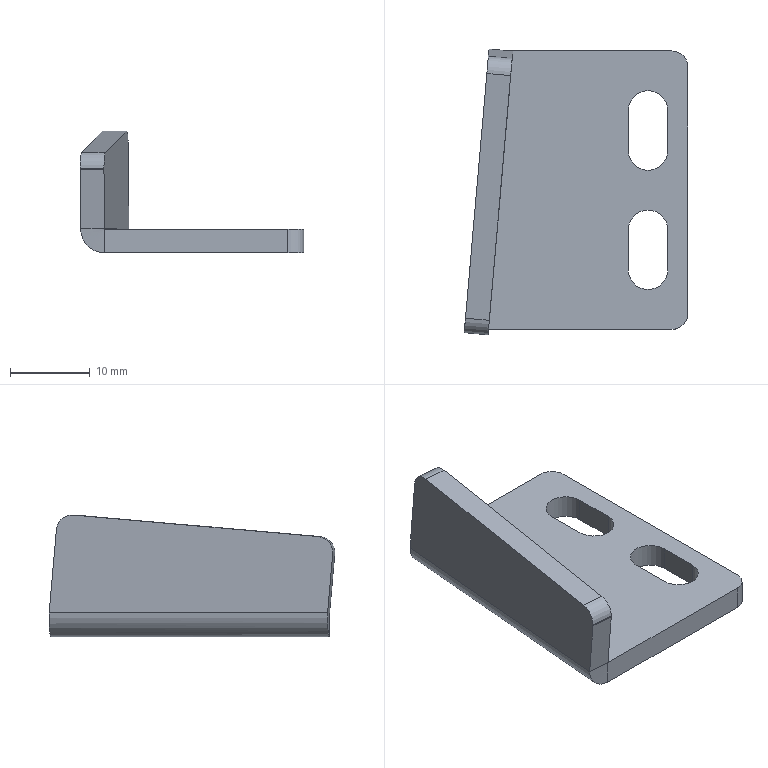Part | NX | features BREP 1 | 1 solid | 27 faces | box 28.112 x 35.918 x 15.317 mm | volume 3596 mm3 | plane 14 | cylinder 11 | spline 2 | commonest cylinder face diameters 4 x5 5 x4 0.02 x1 6.02 x1
STEP:
#1=CARTESIAN_POINT('',(-7.623,-18.197,10.615));
#2=VERTEX_POINT('',#1);
#3=CARTESIAN_POINT('',(-7.622,-18.189,10.441));
#4=VERTEX_POINT('',#3);
#5=CARTESIAN_POINT('',(-7.449,-16.204,10.615));
#6=DIRECTION('',(0.9962,-0.08716,0.));
#7=DIRECTION('',(0.08716,0.9962,0.));
#8=AXIS2_PLACEMENT_3D('',#5,#6,#7);
#9=CIRCLE('',#8,2.);
#10=EDGE_CURVE('',#2,#4,#9,.T.);
#11=ORIENTED_EDGE('',*,*,#10,.F.);
#12=CARTESIAN_POINT('',(-10.612,-17.935,10.615));
#13=VERTEX_POINT('',#12);
#14=CARTESIAN_POINT('',(-7.623,-18.197,10.615));
#15=DIRECTION('',(-0.9962,0.08716,0.));
#16=VECTOR('',#15,1000.);
#17=LINE('',#14,#16);
#18=EDGE_CURVE('',#2,#13,#17,.T.);
#19=ORIENTED_EDGE('',*,*,#18,.T.);
#20=CARTESIAN_POINT('',(-10.611,-17.928,10.441));
#21=VERTEX_POINT('',#20);
#22=CARTESIAN_POINT('',(-10.437,-15.943,10.615));
#23=DIRECTION('',(-0.9962,0.08716,0.));
#24=DIRECTION('',(0.08716,0.9962,0.));
#25=AXIS2_PLACEMENT_3D('',#22,#23,#24);
#26=CIRCLE('',#25,2.);
#27=EDGE_CURVE('',#21,#13,#26,.T.);
#28=ORIENTED_EDGE('',*,*,#27,.F.);
#29=CARTESIAN_POINT('',(-7.622,-18.189,10.441));
#30=DIRECTION('',(-0.9962,0.08716,0.));
#31=VECTOR('',#30,1000.);
#32=LINE('',#29,#31);
#33=EDGE_CURVE('',#4,#21,#32,.T.);
#34=ORIENTED_EDGE('',*,*,#33,.F.);
#35=EDGE_LOOP('',(#11,#19,#28,#34));
#36=FACE_BOUND('',#35,.T.);
#37=CARTESIAN_POINT('',(-7.449,-16.204,10.615));
#38=DIRECTION('',(-0.9962,0.08716,0.));
#39=DIRECTION('',(-0.08716,-0.9962,0.));
#40=AXIS2_PLACEMENT_3D('',#37,#38,#39);
#41=CYLINDRICAL_SURFACE('',#40,2.);
#42=ADVANCED_FACE('',(#36),#41,.T.);
#43=CARTESIAN_POINT('',(-4.504,17.458,3.01));
#44=VERTEX_POINT('',#43);
#45=CARTESIAN_POINT('',(-4.584,16.545,13.491));
#46=VERTEX_POINT('',#45);
#47=CARTESIAN_POINT('',(-4.599,16.371,15.484));
#48=DIRECTION('',(-0.007596,-0.08682,0.9962));
#49=VECTOR('',#48,1000.);
#50=LINE('',#47,#49);
#51=EDGE_CURVE('',#44,#46,#50,.T.);
#52=ORIENTED_EDGE('',*,*,#51,.T.);
#53=CARTESIAN_POINT('',(-4.772,14.386,15.309));
#54=VERTEX_POINT('',#53);
#55=CARTESIAN_POINT('',(-4.757,14.56,13.317));
#56=DIRECTION('',(0.9962,-0.08716,0.));
#57=DIRECTION('',(0.08716,0.9962,0.));
#58=AXIS2_PLACEMENT_3D('',#55,#56,#57);
#59=CIRCLE('',#58,2.);
#60=EDGE_CURVE('',#46,#54,#59,.T.);
#61=ORIENTED_EDGE('',*,*,#60,.T.);
#62=CARTESIAN_POINT('',(-7.464,-16.378,12.607));
#63=VERTEX_POINT('',#62);
#64=CARTESIAN_POINT('',(-4.599,16.371,15.484));
#65=DIRECTION('',(-0.08682,-0.9924,-0.08716));
#66=VECTOR('',#65,1000.);
#67=LINE('',#64,#66);
#68=EDGE_CURVE('',#54,#63,#67,.T.);
#69=ORIENTED_EDGE('',*,*,#68,.T.);
#70=CARTESIAN_POINT('',(-7.449,-16.204,10.615));
#71=DIRECTION('',(0.9962,-0.08716,0.));
#72=DIRECTION('',(0.08716,0.9962,0.));
#73=AXIS2_PLACEMENT_3D('',#70,#71,#72);
#74=CIRCLE('',#73,2.);
#75=EDGE_CURVE('',#63,#2,#74,.T.);
#76=ORIENTED_EDGE('',*,*,#75,.T.);
#77=ORIENTED_EDGE('',*,*,#10,.T.);
#78=CARTESIAN_POINT('',(-7.566,-17.542,3.01));
#79=VERTEX_POINT('',#78);
#80=CARTESIAN_POINT('',(-7.638,-18.363,12.433));
#81=DIRECTION('',(0.007596,0.08682,-0.9962));
#82=VECTOR('',#81,1000.);
#83=LINE('',#80,#82);
#84=EDGE_CURVE('',#4,#79,#83,.T.);
#85=ORIENTED_EDGE('',*,*,#84,.T.);
#86=CARTESIAN_POINT('',(-7.638,-18.363,3.01));
#87=DIRECTION('',(0.08716,0.9962,0.));
#88=VECTOR('',#87,1000.);
#89=LINE('',#86,#88);
#90=EDGE_CURVE('',#79,#44,#89,.T.);
#91=ORIENTED_EDGE('',*,*,#90,.T.);
#92=EDGE_LOOP('',(#52,#61,#69,#76,#77,#85,#91));
#93=FACE_BOUND('',#92,.T.);
#94=CARTESIAN_POINT('',(-7.638,-18.363,12.433));
#95=DIRECTION('',(0.9962,-0.08716,0.));
#96=DIRECTION('',(0.,0.,-1.));
#97=AXIS2_PLACEMENT_3D('',#94,#95,#96);
#98=PLANE('',#97);
#99=ADVANCED_FACE('',(#93),#98,.T.);
#100=ORIENTED_EDGE('',*,*,#68,.F.);
#101=CARTESIAN_POINT('',(-7.761,14.648,15.309));
#102=VERTEX_POINT('',#101);
#103=CARTESIAN_POINT('',(-4.772,14.386,15.309));
#104=DIRECTION('',(-0.9962,0.08716,0.));
#105=VECTOR('',#104,1000.);
#106=LINE('',#103,#105);
#107=EDGE_CURVE('',#54,#102,#106,.T.);
#108=ORIENTED_EDGE('',*,*,#107,.T.);
#109=CARTESIAN_POINT('',(-10.453,-16.117,12.607));
#110=VERTEX_POINT('',#109);
#111=CARTESIAN_POINT('',(-7.587,16.633,15.484));
#112=DIRECTION('',(-0.08682,-0.9924,-0.08716));
#113=VECTOR('',#112,1000.);
#114=LINE('',#111,#113);
#115=EDGE_CURVE('',#102,#110,#114,.T.);
#116=ORIENTED_EDGE('',*,*,#115,.T.);
#117=CARTESIAN_POINT('',(-7.464,-16.378,12.607));
#118=DIRECTION('',(0.9962,-0.08716,0.));
#119=VECTOR('',#118,1000.);
#120=LINE('',#117,#119);
#121=EDGE_CURVE('',#110,#63,#120,.T.);
#122=ORIENTED_EDGE('',*,*,#121,.T.);
#123=EDGE_LOOP('',(#100,#108,#116,#122));
#124=FACE_BOUND('',#123,.T.);
#125=CARTESIAN_POINT('',(-4.599,16.371,15.484));
#126=DIRECTION('',(0.007596,0.08682,-0.9962));
#127=DIRECTION('',(-1.,0.,-0.007625));
#128=AXIS2_PLACEMENT_3D('',#125,#126,#127);
#129=PLANE('',#128);
#130=ADVANCED_FACE('',(#124),#129,.F.);
#131=ORIENTED_EDGE('',*,*,#84,.F.);
#132=ORIENTED_EDGE('',*,*,#33,.T.);
#133=CARTESIAN_POINT('',(-10.554,-17.28,3.01));
#134=VERTEX_POINT('',#133);
#135=CARTESIAN_POINT('',(-10.626,-18.101,12.433));
#136=DIRECTION('',(0.007596,0.08682,-0.9962));
#137=VECTOR('',#136,1000.);
#138=LINE('',#135,#137);
#139=EDGE_CURVE('',#21,#134,#138,.T.);
#140=ORIENTED_EDGE('',*,*,#139,.T.);
#141=CARTESIAN_POINT('',(-7.566,-17.542,3.01));
#142=CARTESIAN_POINT('',(-10.554,-17.28,3.01));
#143=B_SPLINE_CURVE_WITH_KNOTS('',1,(#141,#142),.UNSPECIFIED.,.F.,.F.,(2,2),(0.,1.),.UNSPECIFIED.);
#144=EDGE_CURVE('',#79,#134,#143,.T.);
#145=ORIENTED_EDGE('',*,*,#144,.F.);
#146=EDGE_LOOP('',(#131,#132,#140,#145));
#147=FACE_BOUND('',#146,.T.);
#148=CARTESIAN_POINT('',(-7.638,-18.363,12.433));
#149=DIRECTION('',(0.08682,0.9924,0.08716));
#150=DIRECTION('',(0.7085,0.,-0.7058));
#151=AXIS2_PLACEMENT_3D('',#148,#149,#150);
#152=PLANE('',#151);
#153=ADVANCED_FACE('',(#147),#152,.F.);
#154=CARTESIAN_POINT('',(-7.492,17.72,3.01));
#155=VERTEX_POINT('',#154);
#156=CARTESIAN_POINT('',(-7.572,16.806,13.491));
#157=VERTEX_POINT('',#156);
#158=CARTESIAN_POINT('',(-7.587,16.633,15.484));
#159=DIRECTION('',(-0.007596,-0.08682,0.9962));
#160=VECTOR('',#159,1000.);
#161=LINE('',#158,#160);
#162=EDGE_CURVE('',#155,#157,#161,.T.);
#163=ORIENTED_EDGE('',*,*,#162,.T.);
#164=CARTESIAN_POINT('',(-4.584,16.545,13.491));
#165=DIRECTION('',(0.9962,-0.08716,0.));
#166=VECTOR('',#165,1000.);
#167=LINE('',#164,#166);
#168=EDGE_CURVE('',#157,#46,#167,.T.);
#169=ORIENTED_EDGE('',*,*,#168,.T.);
#170=ORIENTED_EDGE('',*,*,#51,.F.);
#171=CARTESIAN_POINT('',(-7.492,17.72,3.01));
#172=CARTESIAN_POINT('',(-4.504,17.458,3.01));
#173=B_SPLINE_CURVE_WITH_KNOTS('',1,(#171,#172),.UNSPECIFIED.,.F.,.F.,(2,2),(0.,1.),.UNSPECIFIED.);
#174=EDGE_CURVE('',#155,#44,#173,.T.);
#175=ORIENTED_EDGE('',*,*,#174,.F.);
#176=EDGE_LOOP('',(#163,#169,#170,#175));
#177=FACE_BOUND('',#176,.T.);
#178=CARTESIAN_POINT('',(-4.599,16.371,15.484));
#179=DIRECTION('',(-0.08682,-0.9924,-0.08716));
#180=DIRECTION('',(0.,0.08749,-0.9962));
#181=AXIS2_PLACEMENT_3D('',#178,#179,#180);
#182=PLANE('',#181);
#183=ADVANCED_FACE('',(#177),#182,.F.);
#184=ORIENTED_EDGE('',*,*,#115,.F.);
#185=CARTESIAN_POINT('',(-7.746,14.822,13.317));
#186=DIRECTION('',(-0.9962,0.08716,0.));
#187=DIRECTION('',(0.08716,0.9962,0.));
#188=AXIS2_PLACEMENT_3D('',#185,#186,#187);
#189=CIRCLE('',#188,2.);
#190=EDGE_CURVE('',#102,#157,#189,.T.);
#191=ORIENTED_EDGE('',*,*,#190,.T.);
#192=ORIENTED_EDGE('',*,*,#162,.F.);
#193=CARTESIAN_POINT('',(-10.626,-18.101,3.01));
#194=DIRECTION('',(0.08716,0.9962,0.));
#195=VECTOR('',#194,1000.);
#196=LINE('',#193,#195);
#197=EDGE_CURVE('',#134,#155,#196,.T.);
#198=ORIENTED_EDGE('',*,*,#197,.F.);
#199=ORIENTED_EDGE('',*,*,#139,.F.);
#200=ORIENTED_EDGE('',*,*,#27,.T.);
#201=CARTESIAN_POINT('',(-10.437,-15.943,10.615));
#202=DIRECTION('',(-0.9962,0.08716,0.));
#203=DIRECTION('',(0.08716,0.9962,0.));
#204=AXIS2_PLACEMENT_3D('',#201,#202,#203);
#205=CIRCLE('',#204,2.);
#206=EDGE_CURVE('',#13,#110,#205,.T.);
#207=ORIENTED_EDGE('',*,*,#206,.T.);
#208=EDGE_LOOP('',(#184,#191,#192,#198,#199,#200,#207));
#209=FACE_BOUND('',#208,.T.);
#210=CARTESIAN_POINT('',(-10.626,-18.101,12.433));
#211=DIRECTION('',(0.9962,-0.08716,0.));
#212=DIRECTION('',(0.,0.,-1.));
#213=AXIS2_PLACEMENT_3D('',#210,#211,#212);
#214=PLANE('',#213);
#215=ADVANCED_FACE('',(#209),#214,.F.);
#216=CARTESIAN_POINT('',(17.5,-15.5,3.));
#217=VERTEX_POINT('',#216);
#218=CARTESIAN_POINT('',(17.5,15.5,3.));
#219=VERTEX_POINT('',#218);
#220=CARTESIAN_POINT('',(17.5,17.5,3.));
#221=DIRECTION('',(0.,1.,0.));
#222=VECTOR('',#221,1000.);
#223=LINE('',#220,#222);
#224=EDGE_CURVE('',#217,#219,#223,.T.);
#225=ORIENTED_EDGE('',*,*,#224,.F.);
#226=CARTESIAN_POINT('',(17.5,-15.5,0.));
#227=VERTEX_POINT('',#226);
#228=CARTESIAN_POINT('',(17.5,-15.5,3.));
#229=DIRECTION('',(0.,0.,-1.));
#230=VECTOR('',#229,1000.);
#231=LINE('',#228,#230);
#232=EDGE_CURVE('',#217,#227,#231,.T.);
#233=ORIENTED_EDGE('',*,*,#232,.T.);
#234=CARTESIAN_POINT('',(17.5,15.5,0.));
#235=VERTEX_POINT('',#234);
#236=CARTESIAN_POINT('',(17.5,17.5,0.));
#237=DIRECTION('',(0.,1.,0.));
#238=VECTOR('',#237,1000.);
#239=LINE('',#236,#238);
#240=EDGE_CURVE('',#227,#235,#239,.T.);
#241=ORIENTED_EDGE('',*,*,#240,.T.);
#242=CARTESIAN_POINT('',(17.5,15.5,3.));
#243=DIRECTION('',(0.,0.,1.));
#244=VECTOR('',#243,1000.);
#245=LINE('',#242,#244);
#246=EDGE_CURVE('',#235,#219,#245,.T.);
#247=ORIENTED_EDGE('',*,*,#246,.T.);
#248=EDGE_LOOP('',(#225,#233,#241,#247));
#249=FACE_BOUND('',#248,.T.);
#250=CARTESIAN_POINT('',(17.5,17.5,3.));
#251=DIRECTION('',(-1.,0.,0.));
#252=DIRECTION('',(0.,1.,0.));
#253=AXIS2_PLACEMENT_3D('',#250,#251,#252);
#254=PLANE('',#253);
#255=ADVANCED_FACE('',(#249),#254,.F.);
#256=CARTESIAN_POINT('',(-7.552,-17.5,3.));
#257=VERTEX_POINT('',#256);
#258=CARTESIAN_POINT('',(15.5,-17.5,3.));
#259=VERTEX_POINT('',#258);
#260=CARTESIAN_POINT('',(-17.5,-17.5,3.));
#261=DIRECTION('',(1.,0.,0.));
#262=VECTOR('',#261,1000.);
#263=LINE('',#260,#262);
#264=EDGE_CURVE('',#257,#259,#263,.T.);
#265=ORIENTED_EDGE('',*,*,#264,.T.);
#266=CARTESIAN_POINT('',(15.5,-15.5,3.));
#267=DIRECTION('',(0.,0.,1.));
#268=DIRECTION('',(1.,0.,0.));
#269=AXIS2_PLACEMENT_3D('',#266,#267,#268);
#270=CIRCLE('',#269,2.);
#271=EDGE_CURVE('',#259,#217,#270,.T.);
#272=ORIENTED_EDGE('',*,*,#271,.T.);
#273=ORIENTED_EDGE('',*,*,#224,.T.);
#274=CARTESIAN_POINT('',(15.5,17.5,3.));
#275=VERTEX_POINT('',#274);
#276=CARTESIAN_POINT('',(15.5,15.5,3.));
#277=DIRECTION('',(0.,0.,1.));
#278=DIRECTION('',(1.,0.,0.));
#279=AXIS2_PLACEMENT_3D('',#276,#277,#278);
#280=CIRCLE('',#279,2.);
#281=EDGE_CURVE('',#219,#275,#280,.T.);
#282=ORIENTED_EDGE('',*,*,#281,.T.);
#283=CARTESIAN_POINT('',(-4.49,17.5,3.));
#284=VERTEX_POINT('',#283);
#285=CARTESIAN_POINT('',(-17.5,17.5,3.));
#286=DIRECTION('',(-1.,0.,0.));
#287=VECTOR('',#286,1000.);
#288=LINE('',#285,#287);
#289=EDGE_CURVE('',#275,#284,#288,.T.);
#290=ORIENTED_EDGE('',*,*,#289,.T.);
#291=CARTESIAN_POINT('',(-7.628,-18.364,3.));
#292=DIRECTION('',(0.08716,0.9962,0.));
#293=VECTOR('',#292,1000.);
#294=LINE('',#291,#293);
#295=EDGE_CURVE('',#257,#284,#294,.T.);
#296=ORIENTED_EDGE('',*,*,#295,.F.);
#297=EDGE_LOOP('',(#265,#272,#273,#282,#290,#296));
#298=FACE_BOUND('',#297,.T.);
#299=CARTESIAN_POINT('',(15.,-5.,3.));
#300=VERTEX_POINT('',#299);
#301=CARTESIAN_POINT('',(10.,-5.,3.));
#302=VERTEX_POINT('',#301);
#303=CARTESIAN_POINT('',(12.5,-5.,3.));
#304=DIRECTION('',(0.,0.,1.));
#305=DIRECTION('',(-1.,0.,0.));
#306=AXIS2_PLACEMENT_3D('',#303,#304,#305);
#307=CIRCLE('',#306,2.5);
#308=EDGE_CURVE('',#300,#302,#307,.T.);
#309=ORIENTED_EDGE('',*,*,#308,.F.);
#310=CARTESIAN_POINT('',(15.,-10.,3.));
#311=VERTEX_POINT('',#310);
#312=CARTESIAN_POINT('',(15.,-5.,3.));
#313=DIRECTION('',(0.,1.,0.));
#314=VECTOR('',#313,1000.);
#315=LINE('',#312,#314);
#316=EDGE_CURVE('',#311,#300,#315,.T.);
#317=ORIENTED_EDGE('',*,*,#316,.F.);
#318=CARTESIAN_POINT('',(10.,-10.,3.));
#319=VERTEX_POINT('',#318);
#320=CARTESIAN_POINT('',(12.5,-10.,3.));
#321=DIRECTION('',(0.,0.,1.));
#322=DIRECTION('',(-1.,0.,0.));
#323=AXIS2_PLACEMENT_3D('',#320,#321,#322);
#324=CIRCLE('',#323,2.5);
#325=EDGE_CURVE('',#319,#311,#324,.T.);
#326=ORIENTED_EDGE('',*,*,#325,.F.);
#327=CARTESIAN_POINT('',(10.,-10.,3.));
#328=DIRECTION('',(0.,-1.,0.));
#329=VECTOR('',#328,1000.);
#330=LINE('',#327,#329);
#331=EDGE_CURVE('',#302,#319,#330,.T.);
#332=ORIENTED_EDGE('',*,*,#331,.F.);
#333=EDGE_LOOP('',(#309,#317,#326,#332));
#334=FACE_BOUND('',#333,.T.);
#335=CARTESIAN_POINT('',(15.,10.,3.));
#336=VERTEX_POINT('',#335);
#337=CARTESIAN_POINT('',(10.,10.,3.));
#338=VERTEX_POINT('',#337);
#339=CARTESIAN_POINT('',(12.5,10.,3.));
#340=DIRECTION('',(0.,0.,1.));
#341=DIRECTION('',(-1.,0.,0.));
#342=AXIS2_PLACEMENT_3D('',#339,#340,#341);
#343=CIRCLE('',#342,2.5);
#344=EDGE_CURVE('',#336,#338,#343,.T.);
#345=ORIENTED_EDGE('',*,*,#344,.F.);
#346=CARTESIAN_POINT('',(15.,5.,3.));
#347=VERTEX_POINT('',#346);
#348=CARTESIAN_POINT('',(15.,10.,3.));
#349=DIRECTION('',(0.,1.,0.));
#350=VECTOR('',#349,1000.);
#351=LINE('',#348,#350);
#352=EDGE_CURVE('',#347,#336,#351,.T.);
#353=ORIENTED_EDGE('',*,*,#352,.F.);
#354=CARTESIAN_POINT('',(10.,5.,3.));
#355=VERTEX_POINT('',#354);
#356=CARTESIAN_POINT('',(12.5,5.,3.));
#357=DIRECTION('',(0.,0.,1.));
#358=DIRECTION('',(-1.,0.,0.));
#359=AXIS2_PLACEMENT_3D('',#356,#357,#358);
#360=CIRCLE('',#359,2.5);
#361=EDGE_CURVE('',#355,#347,#360,.T.);
#362=ORIENTED_EDGE('',*,*,#361,.F.);
#363=CARTESIAN_POINT('',(10.,5.,3.));
#364=DIRECTION('',(0.,-1.,0.));
#365=VECTOR('',#364,1000.);
#366=LINE('',#363,#365);
#367=EDGE_CURVE('',#338,#355,#366,.T.);
#368=ORIENTED_EDGE('',*,*,#367,.F.);
#369=EDGE_LOOP('',(#345,#353,#362,#368));
#370=FACE_BOUND('',#369,.T.);
#371=CARTESIAN_POINT('',(-17.5,-17.5,3.));
#372=DIRECTION('',(0.,0.,1.));
#373=DIRECTION('',(1.,0.,0.));
#374=AXIS2_PLACEMENT_3D('',#371,#372,#373);
#375=PLANE('',#374);
#376=ADVANCED_FACE('',(#298,#334,#370),#375,.T.);
#377=CARTESIAN_POINT('',(-7.552,-17.5,0.));
#378=VERTEX_POINT('',#377);
#379=CARTESIAN_POINT('',(15.5,-17.5,0.));
#380=VERTEX_POINT('',#379);
#381=CARTESIAN_POINT('',(-17.5,-17.5,0.));
#382=DIRECTION('',(1.,0.,0.));
#383=VECTOR('',#382,1000.);
#384=LINE('',#381,#383);
#385=EDGE_CURVE('',#378,#380,#384,.T.);
#386=ORIENTED_EDGE('',*,*,#385,.T.);
#387=CARTESIAN_POINT('',(15.5,-17.5,3.));
#388=DIRECTION('',(0.,0.,1.));
#389=VECTOR('',#388,1000.);
#390=LINE('',#387,#389);
#391=EDGE_CURVE('',#380,#259,#390,.T.);
#392=ORIENTED_EDGE('',*,*,#391,.T.);
#393=ORIENTED_EDGE('',*,*,#264,.F.);
#394=CARTESIAN_POINT('',(-7.552,-17.5,3.));
#395=CARTESIAN_POINT('',(-7.552,-17.5,2.));
#396=CARTESIAN_POINT('',(-7.552,-17.5,1.));
#397=CARTESIAN_POINT('',(-7.552,-17.5,0.));
#398=B_SPLINE_CURVE_WITH_KNOTS('',3,(#394,#395,#396,#397),.UNSPECIFIED.,.F.,.F.,(4,4),(0.,1.),.UNSPECIFIED.);
#399=EDGE_CURVE('',#257,#378,#398,.T.);
#400=ORIENTED_EDGE('',*,*,#399,.T.);
#401=EDGE_LOOP('',(#386,#392,#393,#400));
#402=FACE_BOUND('',#401,.T.);
#403=CARTESIAN_POINT('',(-17.5,-17.5,3.));
#404=DIRECTION('',(0.,1.,0.));
#405=DIRECTION('',(1.,0.,0.));
#406=AXIS2_PLACEMENT_3D('',#403,#404,#405);
#407=PLANE('',#406);
#408=ADVANCED_FACE('',(#402),#407,.F.);
#409=ORIENTED_EDGE('',*,*,#240,.F.);
#410=CARTESIAN_POINT('',(15.5,-15.5,0.));
#411=DIRECTION('',(0.,0.,-1.));
#412=DIRECTION('',(1.,0.,0.));
#413=AXIS2_PLACEMENT_3D('',#410,#411,#412);
#414=CIRCLE('',#413,2.);
#415=EDGE_CURVE('',#227,#380,#414,.T.);
#416=ORIENTED_EDGE('',*,*,#415,.T.);
#417=ORIENTED_EDGE('',*,*,#385,.F.);
#418=CARTESIAN_POINT('',(-4.49,17.5,-0.000000004));
#419=VERTEX_POINT('',#418);
#420=CARTESIAN_POINT('',(-7.628,-18.364,0.));
#421=DIRECTION('',(0.08716,0.9962,0.));
#422=VECTOR('',#421,1000.);
#423=LINE('',#420,#422);
#424=EDGE_CURVE('',#378,#419,#423,.T.);
#425=ORIENTED_EDGE('',*,*,#424,.T.);
#426=CARTESIAN_POINT('',(15.5,17.5,0.));
#427=VERTEX_POINT('',#426);
#428=CARTESIAN_POINT('',(-17.5,17.5,0.));
#429=DIRECTION('',(-1.,0.,0.));
#430=VECTOR('',#429,1000.);
#431=LINE('',#428,#430);
#432=EDGE_CURVE('',#427,#419,#431,.T.);
#433=ORIENTED_EDGE('',*,*,#432,.F.);
#434=CARTESIAN_POINT('',(15.5,15.5,0.));
#435=DIRECTION('',(0.,0.,-1.));
#436=DIRECTION('',(1.,0.,0.));
#437=AXIS2_PLACEMENT_3D('',#434,#435,#436);
#438=CIRCLE('',#437,2.);
#439=EDGE_CURVE('',#427,#235,#438,.T.);
#440=ORIENTED_EDGE('',*,*,#439,.T.);
#441=EDGE_LOOP('',(#409,#416,#417,#425,#433,#440));
#442=FACE_BOUND('',#441,.T.);
#443=CARTESIAN_POINT('',(15.,-10.,0.));
#444=VERTEX_POINT('',#443);
#445=CARTESIAN_POINT('',(15.,-5.,0.));
#446=VERTEX_POINT('',#445);
#447=CARTESIAN_POINT('',(15.,-17.5,0.));
#448=DIRECTION('',(0.,1.,0.));
#449=VECTOR('',#448,1000.);
#450=LINE('',#447,#449);
#451=EDGE_CURVE('',#444,#446,#450,.T.);
#452=ORIENTED_EDGE('',*,*,#451,.T.);
#453=CARTESIAN_POINT('',(10.,-5.,0.));
#454=VERTEX_POINT('',#453);
#455=CARTESIAN_POINT('',(12.5,-5.,0.));
#456=DIRECTION('',(0.,0.,1.));
#457=DIRECTION('',(1.,0.,0.));
#458=AXIS2_PLACEMENT_3D('',#455,#456,#457);
#459=CIRCLE('',#458,2.5);
#460=EDGE_CURVE('',#446,#454,#459,.T.);
#461=ORIENTED_EDGE('',*,*,#460,.T.);
#462=CARTESIAN_POINT('',(10.,-10.,0.));
#463=VERTEX_POINT('',#462);
#464=CARTESIAN_POINT('',(10.,-17.5,0.));
#465=DIRECTION('',(0.,-1.,0.));
#466=VECTOR('',#465,1000.);
#467=LINE('',#464,#466);
#468=EDGE_CURVE('',#454,#463,#467,.T.);
#469=ORIENTED_EDGE('',*,*,#468,.T.);
#470=CARTESIAN_POINT('',(12.5,-10.,0.));
#471=DIRECTION('',(0.,0.,1.));
#472=DIRECTION('',(1.,0.,0.));
#473=AXIS2_PLACEMENT_3D('',#470,#471,#472);
#474=CIRCLE('',#473,2.5);
#475=EDGE_CURVE('',#463,#444,#474,.T.);
#476=ORIENTED_EDGE('',*,*,#475,.T.);
#477=EDGE_LOOP('',(#452,#461,#469,#476));
#478=FACE_BOUND('',#477,.T.);
#479=CARTESIAN_POINT('',(15.,5.,0.));
#480=VERTEX_POINT('',#479);
#481=CARTESIAN_POINT('',(15.,10.,0.));
#482=VERTEX_POINT('',#481);
#483=CARTESIAN_POINT('',(15.,-17.5,0.));
#484=DIRECTION('',(0.,1.,0.));
#485=VECTOR('',#484,1000.);
#486=LINE('',#483,#485);
#487=EDGE_CURVE('',#480,#482,#486,.T.);
#488=ORIENTED_EDGE('',*,*,#487,.T.);
#489=CARTESIAN_POINT('',(10.,10.,0.));
#490=VERTEX_POINT('',#489);
#491=CARTESIAN_POINT('',(12.5,10.,0.));
#492=DIRECTION('',(0.,0.,1.));
#493=DIRECTION('',(1.,0.,0.));
#494=AXIS2_PLACEMENT_3D('',#491,#492,#493);
#495=CIRCLE('',#494,2.5);
#496=EDGE_CURVE('',#482,#490,#495,.T.);
#497=ORIENTED_EDGE('',*,*,#496,.T.);
#498=CARTESIAN_POINT('',(10.,5.,0.));
#499=VERTEX_POINT('',#498);
#500=CARTESIAN_POINT('',(10.,-17.5,0.));
#501=DIRECTION('',(0.,-1.,0.));
#502=VECTOR('',#501,1000.);
#503=LINE('',#500,#502);
#504=EDGE_CURVE('',#490,#499,#503,.T.);
#505=ORIENTED_EDGE('',*,*,#504,.T.);
#506=CARTESIAN_POINT('',(12.5,5.,0.));
#507=DIRECTION('',(0.,0.,1.));
#508=DIRECTION('',(1.,0.,0.));
#509=AXIS2_PLACEMENT_3D('',#506,#507,#508);
#510=CIRCLE('',#509,2.5);
#511=EDGE_CURVE('',#499,#480,#510,.T.);
#512=ORIENTED_EDGE('',*,*,#511,.T.);
#513=EDGE_LOOP('',(#488,#497,#505,#512));
#514=FACE_BOUND('',#513,.T.);
#515=CARTESIAN_POINT('',(-17.5,-17.5,0.));
#516=DIRECTION('',(0.,0.,1.));
#517=DIRECTION('',(1.,0.,0.));
#518=AXIS2_PLACEMENT_3D('',#515,#516,#517);
#519=PLANE('',#518);
#520=ADVANCED_FACE('',(#442,#478,#514),#519,.F.);
#521=ORIENTED_EDGE('',*,*,#289,.F.);
#522=CARTESIAN_POINT('',(15.5,17.5,3.));
#523=DIRECTION('',(0.,0.,-1.));
#524=VECTOR('',#523,1000.);
#525=LINE('',#522,#524);
#526=EDGE_CURVE('',#275,#427,#525,.T.);
#527=ORIENTED_EDGE('',*,*,#526,.T.);
#528=ORIENTED_EDGE('',*,*,#432,.T.);
#529=CARTESIAN_POINT('',(-4.49,17.5,-0.000000004));
#530=CARTESIAN_POINT('',(-4.49,17.5,1.));
#531=CARTESIAN_POINT('',(-4.49,17.5,2.));
#532=CARTESIAN_POINT('',(-4.49,17.5,3.));
#533=B_SPLINE_CURVE_WITH_KNOTS('',3,(#529,#530,#531,#532),.UNSPECIFIED.,.F.,.F.,(4,4),(0.,1.),.UNSPECIFIED.);
#534=EDGE_CURVE('',#419,#284,#533,.T.);
#535=ORIENTED_EDGE('',*,*,#534,.T.);
#536=EDGE_LOOP('',(#521,#527,#528,#535));
#537=FACE_BOUND('',#536,.T.);
#538=CARTESIAN_POINT('',(-17.5,17.5,3.));
#539=DIRECTION('',(0.,-1.,0.));
#540=DIRECTION('',(0.,0.,-1.));
#541=AXIS2_PLACEMENT_3D('',#538,#539,#540);
#542=PLANE('',#541);
#543=ADVANCED_FACE('',(#537),#542,.F.);
#544=ORIENTED_EDGE('',*,*,#144,.T.);
#545=CARTESIAN_POINT('',(-7.552,-17.5,-0.000000004));
#546=CARTESIAN_POINT('',(-8.338,-17.438,-0.000000004));
#547=CARTESIAN_POINT('',(-9.903,-17.316,0.6522));
#548=CARTESIAN_POINT('',(-10.554,-17.273,2.222));
#549=CARTESIAN_POINT('',(-10.554,-17.28,3.01));
#550=B_SPLINE_CURVE_WITH_KNOTS('',3,(#545,#546,#547,#548,#549),.UNSPECIFIED.,.F.,.F.,(4,1,4),(0.,0.5,1.),.UNSPECIFIED.);
#551=EDGE_CURVE('',#134,#378,#550,.F.);
#552=ORIENTED_EDGE('',*,*,#551,.T.);
#553=ORIENTED_EDGE('',*,*,#399,.F.);
#554=CARTESIAN_POINT('',(-7.566,-17.542,3.01));
#555=CARTESIAN_POINT('',(-7.565,-17.527,3.005));
#556=CARTESIAN_POINT('',(-7.559,-17.514,3.));
#557=CARTESIAN_POINT('',(-7.552,-17.5,3.));
#558=B_SPLINE_CURVE_WITH_KNOTS('',3,(#554,#555,#556,#557),.UNSPECIFIED.,.F.,.F.,(4,4),(0.,1.),.UNSPECIFIED.);
#559=EDGE_CURVE('',#79,#257,#558,.T.);
#560=ORIENTED_EDGE('',*,*,#559,.F.);
#561=EDGE_LOOP('',(#544,#552,#553,#560));
#562=FACE_BOUND('',#561,.T.);
#563=CARTESIAN_POINT('',(-10.554,-17.28,3.01));
#564=CARTESIAN_POINT('',(-10.554,-17.277,2.616));
#565=CARTESIAN_POINT('',(-10.476,-17.28,2.222));
#566=CARTESIAN_POINT('',(-10.175,-17.299,1.494));
#567=CARTESIAN_POINT('',(-9.952,-17.315,1.16));
#568=CARTESIAN_POINT('',(-9.396,-17.357,0.603));
#569=CARTESIAN_POINT('',(-9.063,-17.382,0.3799));
#570=CARTESIAN_POINT('',(-8.338,-17.439,0.07834));
#571=CARTESIAN_POINT('',(-7.945,-17.469,-0.000000004));
#572=CARTESIAN_POINT('',(-7.552,-17.5,-0.000000004));
#573=CARTESIAN_POINT('',(-7.566,-17.542,3.01));
#574=CARTESIAN_POINT('',(-7.565,-17.538,3.009));
#575=CARTESIAN_POINT('',(-7.565,-17.535,3.007));
#576=CARTESIAN_POINT('',(-7.563,-17.528,3.005));
#577=CARTESIAN_POINT('',(-7.562,-17.524,3.004));
#578=CARTESIAN_POINT('',(-7.56,-17.518,3.002));
#579=CARTESIAN_POINT('',(-7.558,-17.514,3.001));
#580=CARTESIAN_POINT('',(-7.555,-17.507,3.));
#581=CARTESIAN_POINT('',(-7.554,-17.504,3.));
#582=CARTESIAN_POINT('',(-7.552,-17.5,3.));
#583=B_SPLINE_SURFACE_WITH_KNOTS('',1,3,((#563,#564,#565,#566,#567,#568,#569,#570,#571,#572),(#573,#574,#575,#576,#577,#578,#579,#580,#581,#582)),.RULED_SURF.,.F.,.F.,.F.,(2,2),(4,2,2,2,4),(0.,1.),(0.,0.25,0.5,0.75,1.),.UNSPECIFIED.);
#584=ADVANCED_FACE('',(#562),#583,.F.);
#585=ORIENTED_EDGE('',*,*,#295,.T.);
#586=CARTESIAN_POINT('',(-4.49,17.5,3.));
#587=CARTESIAN_POINT('',(-4.496,17.486,3.));
#588=CARTESIAN_POINT('',(-4.502,17.473,3.005));
#589=CARTESIAN_POINT('',(-4.504,17.458,3.01));
#590=B_SPLINE_CURVE_WITH_KNOTS('',3,(#586,#587,#588,#589),.UNSPECIFIED.,.F.,.F.,(4,4),(0.,1.),.UNSPECIFIED.);
#591=EDGE_CURVE('',#284,#44,#590,.T.);
#592=ORIENTED_EDGE('',*,*,#591,.T.);
#593=ORIENTED_EDGE('',*,*,#90,.F.);
#594=ORIENTED_EDGE('',*,*,#559,.T.);
#595=EDGE_LOOP('',(#585,#592,#593,#594));
#596=FACE_BOUND('',#595,.T.);
#597=CARTESIAN_POINT('',(-2.944,35.173,3.01));
#598=DIRECTION('',(-0.08716,-0.9962,0.));
#599=DIRECTION('',(0.9962,-0.08716,0.));
#600=AXIS2_PLACEMENT_3D('',#597,#598,#599);
#601=CYLINDRICAL_SURFACE('',#600,0.01);
#602=ADVANCED_FACE('',(#596),#601,.F.);
#603=CARTESIAN_POINT('',(-7.492,17.72,3.01));
#604=CARTESIAN_POINT('',(-7.492,17.727,2.222));
#605=CARTESIAN_POINT('',(-6.841,17.684,0.6522));
#606=CARTESIAN_POINT('',(-5.276,17.562,-0.000000004));
#607=CARTESIAN_POINT('',(-4.49,17.5,-0.000000004));
#608=B_SPLINE_CURVE_WITH_KNOTS('',3,(#603,#604,#605,#606,#607),.UNSPECIFIED.,.F.,.F.,(4,1,4),(0.,0.5,1.),.UNSPECIFIED.);
#609=EDGE_CURVE('',#419,#155,#608,.F.);
#610=ORIENTED_EDGE('',*,*,#609,.T.);
#611=ORIENTED_EDGE('',*,*,#174,.T.);
#612=ORIENTED_EDGE('',*,*,#591,.F.);
#613=ORIENTED_EDGE('',*,*,#534,.F.);
#614=EDGE_LOOP('',(#610,#611,#612,#613));
#615=FACE_BOUND('',#614,.T.);
#616=CARTESIAN_POINT('',(-4.49,17.5,-0.000000004));
#617=CARTESIAN_POINT('',(-4.883,17.531,-0.000000004));
#618=CARTESIAN_POINT('',(-5.275,17.562,0.07834));
#619=CARTESIAN_POINT('',(-6.001,17.618,0.3799));
#620=CARTESIAN_POINT('',(-6.334,17.644,0.603));
#621=CARTESIAN_POINT('',(-6.89,17.685,1.16));
#622=CARTESIAN_POINT('',(-7.112,17.701,1.494));
#623=CARTESIAN_POINT('',(-7.414,17.72,2.222));
#624=CARTESIAN_POINT('',(-7.492,17.724,2.616));
#625=CARTESIAN_POINT('',(-7.492,17.72,3.01));
#626=CARTESIAN_POINT('',(-4.49,17.5,3.));
#627=CARTESIAN_POINT('',(-4.492,17.497,3.));
#628=CARTESIAN_POINT('',(-4.493,17.493,3.));
#629=CARTESIAN_POINT('',(-4.496,17.487,3.001));
#630=CARTESIAN_POINT('',(-4.498,17.483,3.002));
#631=CARTESIAN_POINT('',(-4.5,17.476,3.004));
#632=CARTESIAN_POINT('',(-4.501,17.473,3.005));
#633=CARTESIAN_POINT('',(-4.503,17.466,3.007));
#634=CARTESIAN_POINT('',(-4.503,17.462,3.009));
#635=CARTESIAN_POINT('',(-4.504,17.458,3.01));
#636=B_SPLINE_SURFACE_WITH_KNOTS('',1,3,((#616,#617,#618,#619,#620,#621,#622,#623,#624,#625),(#626,#627,#628,#629,#630,#631,#632,#633,#634,#635)),.RULED_SURF.,.F.,.F.,.F.,(2,2),(4,2,2,2,4),(0.,1.),(0.,0.25,0.5,0.75,1.),.UNSPECIFIED.);
#637=ADVANCED_FACE('',(#615),#636,.F.);
#638=ORIENTED_EDGE('',*,*,#424,.F.);
#639=ORIENTED_EDGE('',*,*,#551,.F.);
#640=ORIENTED_EDGE('',*,*,#197,.T.);
#641=ORIENTED_EDGE('',*,*,#609,.F.);
#642=EDGE_LOOP('',(#638,#639,#640,#641));
#643=FACE_BOUND('',#642,.T.);
#644=CARTESIAN_POINT('',(-2.944,35.173,3.01));
#645=DIRECTION('',(-0.08716,-0.9962,0.));
#646=DIRECTION('',(0.9962,-0.08716,0.));
#647=AXIS2_PLACEMENT_3D('',#644,#645,#646);
#648=CYLINDRICAL_SURFACE('',#647,3.01);
#649=ADVANCED_FACE('',(#643),#648,.T.);
#650=CARTESIAN_POINT('',(15.,10.,-7.));
#651=DIRECTION('',(0.,0.,1.));
#652=VECTOR('',#651,1000.);
#653=LINE('',#650,#652);
#654=EDGE_CURVE('',#482,#336,#653,.T.);
#655=ORIENTED_EDGE('',*,*,#654,.T.);
#656=ORIENTED_EDGE('',*,*,#344,.T.);
#657=CARTESIAN_POINT('',(10.,10.,-7.));
#658=DIRECTION('',(0.,0.,1.));
#659=VECTOR('',#658,1000.);
#660=LINE('',#657,#659);
#661=EDGE_CURVE('',#490,#338,#660,.T.);
#662=ORIENTED_EDGE('',*,*,#661,.F.);
#663=ORIENTED_EDGE('',*,*,#496,.F.);
#664=EDGE_LOOP('',(#655,#656,#662,#663));
#665=FACE_BOUND('',#664,.T.);
#666=CARTESIAN_POINT('',(12.5,10.,-7.));
#667=DIRECTION('',(0.,0.,1.));
#668=DIRECTION('',(1.,0.,0.));
#669=AXIS2_PLACEMENT_3D('',#666,#667,#668);
#670=CYLINDRICAL_SURFACE('',#669,2.5);
#671=ADVANCED_FACE('',(#665),#670,.F.);
#672=CARTESIAN_POINT('',(15.,5.,-7.));
#673=DIRECTION('',(0.,0.,1.));
#674=VECTOR('',#673,1000.);
#675=LINE('',#672,#674);
#676=EDGE_CURVE('',#480,#347,#675,.T.);
#677=ORIENTED_EDGE('',*,*,#676,.T.);
#678=ORIENTED_EDGE('',*,*,#352,.T.);
#679=ORIENTED_EDGE('',*,*,#654,.F.);
#680=ORIENTED_EDGE('',*,*,#487,.F.);
#681=EDGE_LOOP('',(#677,#678,#679,#680));
#682=FACE_BOUND('',#681,.T.);
#683=CARTESIAN_POINT('',(15.,10.,-7.));
#684=DIRECTION('',(1.,0.,0.));
#685=DIRECTION('',(0.,0.,-1.));
#686=AXIS2_PLACEMENT_3D('',#683,#684,#685);
#687=PLANE('',#686);
#688=ADVANCED_FACE('',(#682),#687,.F.);
#689=CARTESIAN_POINT('',(10.,5.,-7.));
#690=DIRECTION('',(0.,0.,1.));
#691=VECTOR('',#690,1000.);
#692=LINE('',#689,#691);
#693=EDGE_CURVE('',#499,#355,#692,.T.);
#694=ORIENTED_EDGE('',*,*,#693,.T.);
#695=ORIENTED_EDGE('',*,*,#361,.T.);
#696=ORIENTED_EDGE('',*,*,#676,.F.);
#697=ORIENTED_EDGE('',*,*,#511,.F.);
#698=EDGE_LOOP('',(#694,#695,#696,#697));
#699=FACE_BOUND('',#698,.T.);
#700=CARTESIAN_POINT('',(12.5,5.,-7.));
#701=DIRECTION('',(0.,0.,1.));
#702=DIRECTION('',(1.,0.,0.));
#703=AXIS2_PLACEMENT_3D('',#700,#701,#702);
#704=CYLINDRICAL_SURFACE('',#703,2.5);
#705=ADVANCED_FACE('',(#699),#704,.F.);
#706=ORIENTED_EDGE('',*,*,#661,.T.);
#707=ORIENTED_EDGE('',*,*,#367,.T.);
#708=ORIENTED_EDGE('',*,*,#693,.F.);
#709=ORIENTED_EDGE('',*,*,#504,.F.);
#710=EDGE_LOOP('',(#706,#707,#708,#709));
#711=FACE_BOUND('',#710,.T.);
#712=CARTESIAN_POINT('',(10.,5.,-7.));
#713=DIRECTION('',(-1.,0.,0.));
#714=DIRECTION('',(0.,1.,0.));
#715=AXIS2_PLACEMENT_3D('',#712,#713,#714);
#716=PLANE('',#715);
#717=ADVANCED_FACE('',(#711),#716,.F.);
#718=CARTESIAN_POINT('',(15.,-5.,-7.));
#719=DIRECTION('',(0.,0.,1.));
#720=VECTOR('',#719,1000.);
#721=LINE('',#718,#720);
#722=EDGE_CURVE('',#446,#300,#721,.T.);
#723=ORIENTED_EDGE('',*,*,#722,.T.);
#724=ORIENTED_EDGE('',*,*,#308,.T.);
#725=CARTESIAN_POINT('',(10.,-5.,-7.));
#726=DIRECTION('',(0.,0.,1.));
#727=VECTOR('',#726,1000.);
#728=LINE('',#725,#727);
#729=EDGE_CURVE('',#454,#302,#728,.T.);
#730=ORIENTED_EDGE('',*,*,#729,.F.);
#731=ORIENTED_EDGE('',*,*,#460,.F.);
#732=EDGE_LOOP('',(#723,#724,#730,#731));
#733=FACE_BOUND('',#732,.T.);
#734=CARTESIAN_POINT('',(12.5,-5.,-7.));
#735=DIRECTION('',(0.,0.,1.));
#736=DIRECTION('',(1.,0.,0.));
#737=AXIS2_PLACEMENT_3D('',#734,#735,#736);
#738=CYLINDRICAL_SURFACE('',#737,2.5);
#739=ADVANCED_FACE('',(#733),#738,.F.);
#740=CARTESIAN_POINT('',(15.,-10.,-7.));
#741=DIRECTION('',(0.,0.,1.));
#742=VECTOR('',#741,1000.);
#743=LINE('',#740,#742);
#744=EDGE_CURVE('',#444,#311,#743,.T.);
#745=ORIENTED_EDGE('',*,*,#744,.T.);
#746=ORIENTED_EDGE('',*,*,#316,.T.);
#747=ORIENTED_EDGE('',*,*,#722,.F.);
#748=ORIENTED_EDGE('',*,*,#451,.F.);
#749=EDGE_LOOP('',(#745,#746,#747,#748));
#750=FACE_BOUND('',#749,.T.);
#751=CARTESIAN_POINT('',(15.,-5.,-7.));
#752=DIRECTION('',(1.,0.,0.));
#753=DIRECTION('',(0.,0.,-1.));
#754=AXIS2_PLACEMENT_3D('',#751,#752,#753);
#755=PLANE('',#754);
#756=ADVANCED_FACE('',(#750),#755,.F.);
#757=CARTESIAN_POINT('',(10.,-10.,-7.));
#758=DIRECTION('',(0.,0.,1.));
#759=VECTOR('',#758,1000.);
#760=LINE('',#757,#759);
#761=EDGE_CURVE('',#463,#319,#760,.T.);
#762=ORIENTED_EDGE('',*,*,#761,.T.);
#763=ORIENTED_EDGE('',*,*,#325,.T.);
#764=ORIENTED_EDGE('',*,*,#744,.F.);
#765=ORIENTED_EDGE('',*,*,#475,.F.);
#766=EDGE_LOOP('',(#762,#763,#764,#765));
#767=FACE_BOUND('',#766,.T.);
#768=CARTESIAN_POINT('',(12.5,-10.,-7.));
#769=DIRECTION('',(0.,0.,1.));
#770=DIRECTION('',(1.,0.,0.));
#771=AXIS2_PLACEMENT_3D('',#768,#769,#770);
#772=CYLINDRICAL_SURFACE('',#771,2.5);
#773=ADVANCED_FACE('',(#767),#772,.F.);
#774=ORIENTED_EDGE('',*,*,#729,.T.);
#775=ORIENTED_EDGE('',*,*,#331,.T.);
#776=ORIENTED_EDGE('',*,*,#761,.F.);
#777=ORIENTED_EDGE('',*,*,#468,.F.);
#778=EDGE_LOOP('',(#774,#775,#776,#777));
#779=FACE_BOUND('',#778,.T.);
#780=CARTESIAN_POINT('',(10.,-10.,-7.));
#781=DIRECTION('',(-1.,0.,0.));
#782=DIRECTION('',(0.,1.,0.));
#783=AXIS2_PLACEMENT_3D('',#780,#781,#782);
#784=PLANE('',#783);
#785=ADVANCED_FACE('',(#779),#784,.F.);
#786=ORIENTED_EDGE('',*,*,#60,.F.);
#787=ORIENTED_EDGE('',*,*,#168,.F.);
#788=ORIENTED_EDGE('',*,*,#190,.F.);
#789=ORIENTED_EDGE('',*,*,#107,.F.);
#790=EDGE_LOOP('',(#786,#787,#788,#789));
#791=FACE_BOUND('',#790,.T.);
#792=CARTESIAN_POINT('',(-4.757,14.56,13.317));
#793=DIRECTION('',(-0.9962,0.08716,0.));
#794=DIRECTION('',(-0.08716,-0.9962,0.));
#795=AXIS2_PLACEMENT_3D('',#792,#793,#794);
#796=CYLINDRICAL_SURFACE('',#795,2.);
#797=ADVANCED_FACE('',(#791),#796,.T.);
#798=ORIENTED_EDGE('',*,*,#18,.F.);
#799=ORIENTED_EDGE('',*,*,#75,.F.);
#800=ORIENTED_EDGE('',*,*,#121,.F.);
#801=ORIENTED_EDGE('',*,*,#206,.F.);
#802=EDGE_LOOP('',(#798,#799,#800,#801));
#803=FACE_BOUND('',#802,.T.);
#804=CARTESIAN_POINT('',(-7.449,-16.204,10.615));
#805=DIRECTION('',(-0.9962,0.08716,0.));
#806=DIRECTION('',(-0.08716,-0.9962,0.));
#807=AXIS2_PLACEMENT_3D('',#804,#805,#806);
#808=CYLINDRICAL_SURFACE('',#807,2.);
#809=ADVANCED_FACE('',(#803),#808,.T.);
#810=ORIENTED_EDGE('',*,*,#271,.F.);
#811=ORIENTED_EDGE('',*,*,#391,.F.);
#812=ORIENTED_EDGE('',*,*,#415,.F.);
#813=ORIENTED_EDGE('',*,*,#232,.F.);
#814=EDGE_LOOP('',(#810,#811,#812,#813));
#815=FACE_BOUND('',#814,.T.);
#816=CARTESIAN_POINT('',(15.5,-15.5,3.));
#817=DIRECTION('',(0.,0.,-1.));
#818=DIRECTION('',(-1.,0.,0.));
#819=AXIS2_PLACEMENT_3D('',#816,#817,#818);
#820=CYLINDRICAL_SURFACE('',#819,2.);
#821=ADVANCED_FACE('',(#815),#820,.T.);
#822=ORIENTED_EDGE('',*,*,#281,.F.);
#823=ORIENTED_EDGE('',*,*,#246,.F.);
#824=ORIENTED_EDGE('',*,*,#439,.F.);
#825=ORIENTED_EDGE('',*,*,#526,.F.);
#826=EDGE_LOOP('',(#822,#823,#824,#825));
#827=FACE_BOUND('',#826,.T.);
#828=CARTESIAN_POINT('',(15.5,15.5,3.));
#829=DIRECTION('',(0.,0.,-1.));
#830=DIRECTION('',(-1.,0.,0.));
#831=AXIS2_PLACEMENT_3D('',#828,#829,#830);
#832=CYLINDRICAL_SURFACE('',#831,2.);
#833=ADVANCED_FACE('',(#827),#832,.T.);
#834=CLOSED_SHELL('',(#42,#99,#130,#153,#183,#215,#255,#376,#408,#520,#543,#584,#602,#637,#649,#671,#688,#705,#717,#739,#756,#773,#785,#797,#809,#821,#833));
#835=MANIFOLD_SOLID_BREP('',#834);
#836=(LENGTH_UNIT()NAMED_UNIT(*)SI_UNIT(.MILLI.,.METRE.));
#837=UNCERTAINTY_MEASURE_WITH_UNIT(LENGTH_MEASURE(0.0508),#836,'','');
#838=(NAMED_UNIT(*)PLANE_ANGLE_UNIT()SI_UNIT($,.RADIAN.));
#839=(NAMED_UNIT(*)SI_UNIT($,.STERADIAN.)SOLID_ANGLE_UNIT());
#840=(GEOMETRIC_REPRESENTATION_CONTEXT(3)GLOBAL_UNCERTAINTY_ASSIGNED_CONTEXT((#837))GLOBAL_UNIT_ASSIGNED_CONTEXT((#836,#838,#839))REPRESENTATION_CONTEXT('',''));
#841=ADVANCED_BREP_SHAPE_REPRESENTATION('',(#835),#840);